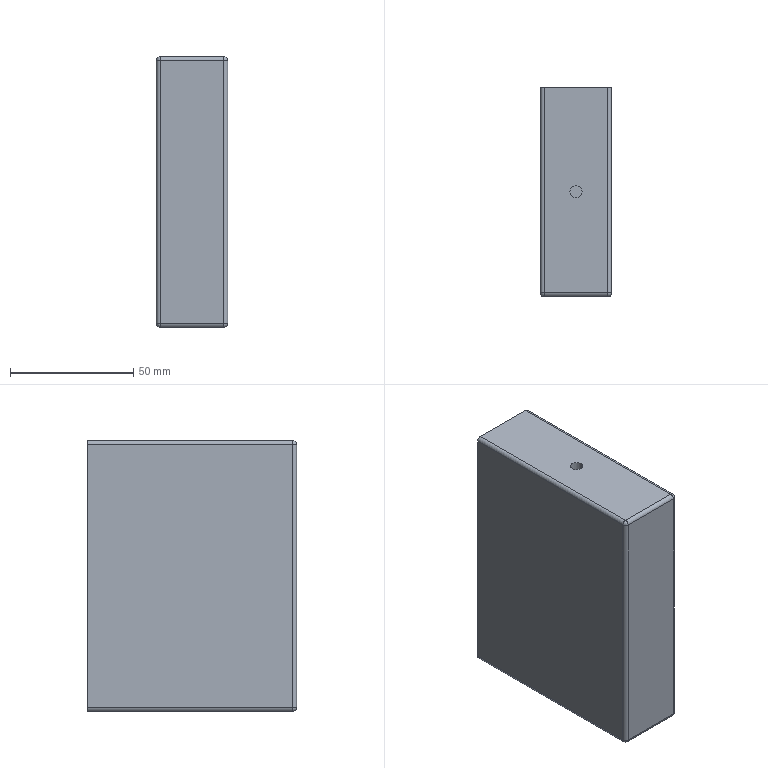Part | SolidWorks | features Extrusion 1, Fillet 1, HoleWzd 1, ICE 1, Shell 1 | 1 solid | 40 faces | box 29 x 85 x 110 mm | volume 26099 mm3 | cylinder 20 | plane 12 | sphere 8 | commonest cylinder face diameters 1 x8 3 x8 5 x2 10 x2
STEP:
#1=CARTESIAN_POINT('',(2.5,0.,51.));
#2=VERTEX_POINT('',#1);
#3=CARTESIAN_POINT('',(-2.5,0.,51.));
#4=VERTEX_POINT('',#3);
#5=CARTESIAN_POINT('',(0.,0.,51.));
#6=DIRECTION('',(0.,0.,-1.));
#7=DIRECTION('',(-1.,0.,0.));
#8=AXIS2_PLACEMENT_3D('',#5,#6,#7);
#9=CIRCLE('',#8,2.5);
#10=EDGE_CURVE('',#2,#4,#9,.T.);
#11=ORIENTED_EDGE('',*,*,#10,.T.);
#12=CARTESIAN_POINT('',(-2.5,0.,55.));
#13=VERTEX_POINT('',#12);
#14=CARTESIAN_POINT('',(-2.5,0.,55.));
#15=DIRECTION('',(0.,0.,1.));
#16=VECTOR('',#15,1000.);
#17=LINE('',#14,#16);
#18=EDGE_CURVE('',#4,#13,#17,.T.);
#19=ORIENTED_EDGE('',*,*,#18,.T.);
#20=CARTESIAN_POINT('',(2.5,0.,55.));
#21=VERTEX_POINT('',#20);
#22=CARTESIAN_POINT('',(0.,0.,55.));
#23=DIRECTION('',(0.,0.,1.));
#24=DIRECTION('',(1.,0.,0.));
#25=AXIS2_PLACEMENT_3D('',#22,#23,#24);
#26=CIRCLE('',#25,2.5);
#27=EDGE_CURVE('',#13,#21,#26,.T.);
#28=ORIENTED_EDGE('',*,*,#27,.T.);
#29=CARTESIAN_POINT('',(2.5,0.,55.));
#30=DIRECTION('',(0.,0.,1.));
#31=VECTOR('',#30,1000.);
#32=LINE('',#29,#31);
#33=EDGE_CURVE('',#2,#21,#32,.T.);
#34=ORIENTED_EDGE('',*,*,#33,.F.);
#35=EDGE_LOOP('',(#11,#19,#28,#34));
#36=FACE_OUTER_BOUND('',#35,.T.);
#37=CARTESIAN_POINT('',(0.,0.,55.));
#38=DIRECTION('',(0.,0.,1.));
#39=DIRECTION('',(1.,0.,0.));
#40=AXIS2_PLACEMENT_3D('',#37,#38,#39);
#41=CYLINDRICAL_SURFACE('',#40,2.5);
#42=ADVANCED_FACE('',(#36),#41,.F.);
#43=CARTESIAN_POINT('',(-5.,0.,51.));
#44=VERTEX_POINT('',#43);
#45=CARTESIAN_POINT('',(5.,0.,51.));
#46=VERTEX_POINT('',#45);
#47=CARTESIAN_POINT('',(0.,0.,51.));
#48=DIRECTION('',(0.,0.,-1.));
#49=DIRECTION('',(-1.,0.,0.));
#50=AXIS2_PLACEMENT_3D('',#47,#48,#49);
#51=CIRCLE('',#50,5.);
#52=EDGE_CURVE('',#44,#46,#51,.T.);
#53=ORIENTED_EDGE('',*,*,#52,.F.);
#54=CARTESIAN_POINT('',(-5.,0.,54.));
#55=VERTEX_POINT('',#54);
#56=CARTESIAN_POINT('',(-5.,0.,51.));
#57=DIRECTION('',(0.,0.,1.));
#58=VECTOR('',#57,1000.);
#59=LINE('',#56,#58);
#60=EDGE_CURVE('',#44,#55,#59,.T.);
#61=ORIENTED_EDGE('',*,*,#60,.T.);
#62=CARTESIAN_POINT('',(5.,0.,54.));
#63=VERTEX_POINT('',#62);
#64=CARTESIAN_POINT('',(0.,0.,54.));
#65=DIRECTION('',(0.,0.,-1.));
#66=DIRECTION('',(-1.,0.,0.));
#67=AXIS2_PLACEMENT_3D('',#64,#65,#66);
#68=CIRCLE('',#67,5.);
#69=EDGE_CURVE('',#55,#63,#68,.T.);
#70=ORIENTED_EDGE('',*,*,#69,.T.);
#71=CARTESIAN_POINT('',(5.,0.,51.));
#72=DIRECTION('',(0.,0.,1.));
#73=VECTOR('',#72,1000.);
#74=LINE('',#71,#73);
#75=EDGE_CURVE('',#46,#63,#74,.T.);
#76=ORIENTED_EDGE('',*,*,#75,.F.);
#77=EDGE_LOOP('',(#53,#61,#70,#76));
#78=FACE_OUTER_BOUND('',#77,.T.);
#79=CARTESIAN_POINT('',(0.,0.,51.));
#80=DIRECTION('',(0.,0.,1.));
#81=DIRECTION('',(1.,0.,0.));
#82=AXIS2_PLACEMENT_3D('',#79,#80,#81);
#83=CYLINDRICAL_SURFACE('',#82,5.);
#84=ADVANCED_FACE('',(#78),#83,.T.);
#85=CARTESIAN_POINT('',(-13.,-41.,54.));
#86=VERTEX_POINT('',#85);
#87=CARTESIAN_POINT('',(13.,-41.,54.));
#88=VERTEX_POINT('',#87);
#89=CARTESIAN_POINT('',(-14.5,-41.,54.));
#90=DIRECTION('',(1.,0.,0.));
#91=VECTOR('',#90,1000.);
#92=LINE('',#89,#91);
#93=EDGE_CURVE('',#86,#88,#92,.T.);
#94=ORIENTED_EDGE('',*,*,#93,.F.);
#95=CARTESIAN_POINT('',(-13.,42.5,54.));
#96=VERTEX_POINT('',#95);
#97=CARTESIAN_POINT('',(-13.,42.5,54.));
#98=DIRECTION('',(0.,-1.,0.));
#99=VECTOR('',#98,1000.);
#100=LINE('',#97,#99);
#101=EDGE_CURVE('',#96,#86,#100,.T.);
#102=ORIENTED_EDGE('',*,*,#101,.F.);
#103=CARTESIAN_POINT('',(13.,42.5,54.));
#104=VERTEX_POINT('',#103);
#105=CARTESIAN_POINT('',(-14.5,42.5,54.));
#106=DIRECTION('',(1.,0.,0.));
#107=VECTOR('',#106,1000.);
#108=LINE('',#105,#107);
#109=EDGE_CURVE('',#96,#104,#108,.T.);
#110=ORIENTED_EDGE('',*,*,#109,.T.);
#111=CARTESIAN_POINT('',(13.,42.5,54.));
#112=DIRECTION('',(0.,1.,0.));
#113=VECTOR('',#112,1000.);
#114=LINE('',#111,#113);
#115=EDGE_CURVE('',#88,#104,#114,.T.);
#116=ORIENTED_EDGE('',*,*,#115,.F.);
#117=EDGE_LOOP('',(#94,#102,#110,#116));
#118=FACE_OUTER_BOUND('',#117,.T.);
#119=CARTESIAN_POINT('',(0.,0.,54.));
#120=DIRECTION('',(0.,0.,-1.));
#121=DIRECTION('',(-1.,0.,0.));
#122=AXIS2_PLACEMENT_3D('',#119,#120,#121);
#123=CIRCLE('',#122,5.);
#124=EDGE_CURVE('',#63,#55,#123,.T.);
#125=ORIENTED_EDGE('',*,*,#124,.F.);
#126=ORIENTED_EDGE('',*,*,#69,.F.);
#127=EDGE_LOOP('',(#125,#126));
#128=FACE_BOUND('',#127,.T.);
#129=CARTESIAN_POINT('',(-14.5,42.5,54.));
#130=DIRECTION('',(0.,0.,-1.));
#131=DIRECTION('',(-1.,0.,0.));
#132=AXIS2_PLACEMENT_3D('',#129,#130,#131);
#133=PLANE('',#132);
#134=ADVANCED_FACE('',(#118,#128),#133,.T.);
#135=CARTESIAN_POINT('',(14.5,-41.,53.5));
#136=VERTEX_POINT('',#135);
#137=CARTESIAN_POINT('',(14.5,-41.,-53.5));
#138=VERTEX_POINT('',#137);
#139=CARTESIAN_POINT('',(14.5,-41.,-55.));
#140=DIRECTION('',(0.,0.,-1.));
#141=VECTOR('',#140,1000.);
#142=LINE('',#139,#141);
#143=EDGE_CURVE('',#136,#138,#142,.T.);
#144=ORIENTED_EDGE('',*,*,#143,.T.);
#145=CARTESIAN_POINT('',(14.5,42.5,-53.5));
#146=VERTEX_POINT('',#145);
#147=CARTESIAN_POINT('',(14.5,42.5,-53.5));
#148=DIRECTION('',(0.,1.,0.));
#149=VECTOR('',#148,1000.);
#150=LINE('',#147,#149);
#151=EDGE_CURVE('',#138,#146,#150,.T.);
#152=ORIENTED_EDGE('',*,*,#151,.T.);
#153=CARTESIAN_POINT('',(14.5,42.5,53.5));
#154=VERTEX_POINT('',#153);
#155=CARTESIAN_POINT('',(14.5,42.5,-55.));
#156=DIRECTION('',(0.,0.,-1.));
#157=VECTOR('',#156,1000.);
#158=LINE('',#155,#157);
#159=EDGE_CURVE('',#154,#146,#158,.T.);
#160=ORIENTED_EDGE('',*,*,#159,.F.);
#161=CARTESIAN_POINT('',(14.5,42.5,53.5));
#162=DIRECTION('',(0.,-1.,0.));
#163=VECTOR('',#162,1000.);
#164=LINE('',#161,#163);
#165=EDGE_CURVE('',#154,#136,#164,.T.);
#166=ORIENTED_EDGE('',*,*,#165,.T.);
#167=EDGE_LOOP('',(#144,#152,#160,#166));
#168=FACE_OUTER_BOUND('',#167,.T.);
#169=CARTESIAN_POINT('',(14.5,42.5,-55.));
#170=DIRECTION('',(-1.,0.,0.));
#171=DIRECTION('',(0.,0.,1.));
#172=AXIS2_PLACEMENT_3D('',#169,#170,#171);
#173=PLANE('',#172);
#174=ADVANCED_FACE('',(#168),#173,.F.);
#175=CARTESIAN_POINT('',(13.,-41.,-55.));
#176=VERTEX_POINT('',#175);
#177=CARTESIAN_POINT('',(-13.,-41.,-55.));
#178=VERTEX_POINT('',#177);
#179=CARTESIAN_POINT('',(-14.5,-41.,-55.));
#180=DIRECTION('',(-1.,0.,0.));
#181=VECTOR('',#180,1000.);
#182=LINE('',#179,#181);
#183=EDGE_CURVE('',#176,#178,#182,.T.);
#184=ORIENTED_EDGE('',*,*,#183,.T.);
#185=CARTESIAN_POINT('',(-13.,42.5,-55.));
#186=VERTEX_POINT('',#185);
#187=CARTESIAN_POINT('',(-13.,42.5,-55.));
#188=DIRECTION('',(0.,1.,0.));
#189=VECTOR('',#188,1000.);
#190=LINE('',#187,#189);
#191=EDGE_CURVE('',#178,#186,#190,.T.);
#192=ORIENTED_EDGE('',*,*,#191,.T.);
#193=CARTESIAN_POINT('',(13.,42.5,-55.));
#194=VERTEX_POINT('',#193);
#195=CARTESIAN_POINT('',(-14.5,42.5,-55.));
#196=DIRECTION('',(-1.,0.,0.));
#197=VECTOR('',#196,1000.);
#198=LINE('',#195,#197);
#199=EDGE_CURVE('',#194,#186,#198,.T.);
#200=ORIENTED_EDGE('',*,*,#199,.F.);
#201=CARTESIAN_POINT('',(13.,42.5,-55.));
#202=DIRECTION('',(0.,-1.,0.));
#203=VECTOR('',#202,1000.);
#204=LINE('',#201,#203);
#205=EDGE_CURVE('',#194,#176,#204,.T.);
#206=ORIENTED_EDGE('',*,*,#205,.T.);
#207=EDGE_LOOP('',(#184,#192,#200,#206));
#208=FACE_OUTER_BOUND('',#207,.T.);
#209=CARTESIAN_POINT('',(-14.5,42.5,-55.));
#210=DIRECTION('',(0.,0.,1.));
#211=DIRECTION('',(1.,0.,0.));
#212=AXIS2_PLACEMENT_3D('',#209,#210,#211);
#213=PLANE('',#212);
#214=ADVANCED_FACE('',(#208),#213,.F.);
#215=CARTESIAN_POINT('',(-14.5,42.5,-53.5));
#216=VERTEX_POINT('',#215);
#217=CARTESIAN_POINT('',(-14.5,42.5,53.5));
#218=VERTEX_POINT('',#217);
#219=CARTESIAN_POINT('',(-14.5,42.5,-55.));
#220=DIRECTION('',(0.,0.,1.));
#221=VECTOR('',#220,1000.);
#222=LINE('',#219,#221);
#223=EDGE_CURVE('',#216,#218,#222,.T.);
#224=ORIENTED_EDGE('',*,*,#223,.F.);
#225=CARTESIAN_POINT('',(-14.5,-41.,-53.5));
#226=VERTEX_POINT('',#225);
#227=CARTESIAN_POINT('',(-14.5,42.5,-53.5));
#228=DIRECTION('',(0.,-1.,0.));
#229=VECTOR('',#228,1000.);
#230=LINE('',#227,#229);
#231=EDGE_CURVE('',#216,#226,#230,.T.);
#232=ORIENTED_EDGE('',*,*,#231,.T.);
#233=CARTESIAN_POINT('',(-14.5,-41.,53.5));
#234=VERTEX_POINT('',#233);
#235=CARTESIAN_POINT('',(-14.5,-41.,-55.));
#236=DIRECTION('',(0.,0.,1.));
#237=VECTOR('',#236,1000.);
#238=LINE('',#235,#237);
#239=EDGE_CURVE('',#226,#234,#238,.T.);
#240=ORIENTED_EDGE('',*,*,#239,.T.);
#241=CARTESIAN_POINT('',(-14.5,42.5,53.5));
#242=DIRECTION('',(0.,1.,0.));
#243=VECTOR('',#242,1000.);
#244=LINE('',#241,#243);
#245=EDGE_CURVE('',#234,#218,#244,.T.);
#246=ORIENTED_EDGE('',*,*,#245,.T.);
#247=EDGE_LOOP('',(#224,#232,#240,#246));
#248=FACE_OUTER_BOUND('',#247,.T.);
#249=CARTESIAN_POINT('',(-14.5,42.5,-55.));
#250=DIRECTION('',(1.,0.,0.));
#251=DIRECTION('',(0.,0.,-1.));
#252=AXIS2_PLACEMENT_3D('',#249,#250,#251);
#253=PLANE('',#252);
#254=ADVANCED_FACE('',(#248),#253,.F.);
#255=CARTESIAN_POINT('',(0.,0.,55.));
#256=DIRECTION('',(0.,0.,1.));
#257=DIRECTION('',(1.,0.,0.));
#258=AXIS2_PLACEMENT_3D('',#255,#256,#257);
#259=CIRCLE('',#258,2.5);
#260=EDGE_CURVE('',#21,#13,#259,.T.);
#261=ORIENTED_EDGE('',*,*,#260,.F.);
#262=ORIENTED_EDGE('',*,*,#27,.F.);
#263=EDGE_LOOP('',(#261,#262));
#264=FACE_BOUND('',#263,.T.);
#265=CARTESIAN_POINT('',(-13.,-41.,55.));
#266=VERTEX_POINT('',#265);
#267=CARTESIAN_POINT('',(13.,-41.,55.));
#268=VERTEX_POINT('',#267);
#269=CARTESIAN_POINT('',(-14.5,-41.,55.));
#270=DIRECTION('',(1.,0.,0.));
#271=VECTOR('',#270,1000.);
#272=LINE('',#269,#271);
#273=EDGE_CURVE('',#266,#268,#272,.T.);
#274=ORIENTED_EDGE('',*,*,#273,.T.);
#275=CARTESIAN_POINT('',(13.,42.5,55.));
#276=VERTEX_POINT('',#275);
#277=CARTESIAN_POINT('',(13.,42.5,55.));
#278=DIRECTION('',(0.,1.,0.));
#279=VECTOR('',#278,1000.);
#280=LINE('',#277,#279);
#281=EDGE_CURVE('',#268,#276,#280,.T.);
#282=ORIENTED_EDGE('',*,*,#281,.T.);
#283=CARTESIAN_POINT('',(-13.,42.5,55.));
#284=VERTEX_POINT('',#283);
#285=CARTESIAN_POINT('',(-14.5,42.5,55.));
#286=DIRECTION('',(1.,0.,0.));
#287=VECTOR('',#286,1000.);
#288=LINE('',#285,#287);
#289=EDGE_CURVE('',#284,#276,#288,.T.);
#290=ORIENTED_EDGE('',*,*,#289,.F.);
#291=CARTESIAN_POINT('',(-13.,42.5,55.));
#292=DIRECTION('',(0.,-1.,0.));
#293=VECTOR('',#292,1000.);
#294=LINE('',#291,#293);
#295=EDGE_CURVE('',#284,#266,#294,.T.);
#296=ORIENTED_EDGE('',*,*,#295,.T.);
#297=EDGE_LOOP('',(#274,#282,#290,#296));
#298=FACE_OUTER_BOUND('',#297,.T.);
#299=CARTESIAN_POINT('',(-14.5,42.5,55.));
#300=DIRECTION('',(0.,0.,-1.));
#301=DIRECTION('',(-1.,0.,0.));
#302=AXIS2_PLACEMENT_3D('',#299,#300,#301);
#303=PLANE('',#302);
#304=ADVANCED_FACE('',(#264,#298),#303,.F.);
#305=CARTESIAN_POINT('',(13.,42.5,-54.));
#306=VERTEX_POINT('',#305);
#307=CARTESIAN_POINT('',(-13.,42.5,-54.));
#308=VERTEX_POINT('',#307);
#309=CARTESIAN_POINT('',(-14.5,42.5,-54.));
#310=DIRECTION('',(-1.,0.,0.));
#311=VECTOR('',#310,1000.);
#312=LINE('',#309,#311);
#313=EDGE_CURVE('',#306,#308,#312,.T.);
#314=ORIENTED_EDGE('',*,*,#313,.F.);
#315=CARTESIAN_POINT('',(13.5,42.5,-53.5));
#316=VERTEX_POINT('',#315);
#317=CARTESIAN_POINT('',(13.,42.5,-53.5));
#318=DIRECTION('',(0.,1.,0.));
#319=DIRECTION('',(0.,0.,1.));
#320=AXIS2_PLACEMENT_3D('',#317,#318,#319);
#321=CIRCLE('',#320,0.5);
#322=EDGE_CURVE('',#316,#306,#321,.T.);
#323=ORIENTED_EDGE('',*,*,#322,.F.);
#324=CARTESIAN_POINT('',(13.5,42.5,53.5));
#325=VERTEX_POINT('',#324);
#326=CARTESIAN_POINT('',(13.5,42.5,-55.));
#327=DIRECTION('',(0.,0.,-1.));
#328=VECTOR('',#327,1000.);
#329=LINE('',#326,#328);
#330=EDGE_CURVE('',#325,#316,#329,.T.);
#331=ORIENTED_EDGE('',*,*,#330,.F.);
#332=CARTESIAN_POINT('',(13.,42.5,53.5));
#333=DIRECTION('',(0.,1.,0.));
#334=DIRECTION('',(0.,0.,1.));
#335=AXIS2_PLACEMENT_3D('',#332,#333,#334);
#336=CIRCLE('',#335,0.5);
#337=EDGE_CURVE('',#104,#325,#336,.T.);
#338=ORIENTED_EDGE('',*,*,#337,.F.);
#339=ORIENTED_EDGE('',*,*,#109,.F.);
#340=CARTESIAN_POINT('',(-13.5,42.5,53.5));
#341=VERTEX_POINT('',#340);
#342=CARTESIAN_POINT('',(-13.,42.5,53.5));
#343=DIRECTION('',(0.,1.,0.));
#344=DIRECTION('',(0.,0.,1.));
#345=AXIS2_PLACEMENT_3D('',#342,#343,#344);
#346=CIRCLE('',#345,0.5);
#347=EDGE_CURVE('',#341,#96,#346,.T.);
#348=ORIENTED_EDGE('',*,*,#347,.F.);
#349=CARTESIAN_POINT('',(-13.5,42.5,-53.5));
#350=VERTEX_POINT('',#349);
#351=CARTESIAN_POINT('',(-13.5,42.5,-55.));
#352=DIRECTION('',(0.,0.,1.));
#353=VECTOR('',#352,1000.);
#354=LINE('',#351,#353);
#355=EDGE_CURVE('',#350,#341,#354,.T.);
#356=ORIENTED_EDGE('',*,*,#355,.F.);
#357=CARTESIAN_POINT('',(-13.,42.5,-53.5));
#358=DIRECTION('',(0.,1.,0.));
#359=DIRECTION('',(0.,0.,1.));
#360=AXIS2_PLACEMENT_3D('',#357,#358,#359);
#361=CIRCLE('',#360,0.5);
#362=EDGE_CURVE('',#308,#350,#361,.T.);
#363=ORIENTED_EDGE('',*,*,#362,.F.);
#364=EDGE_LOOP('',(#314,#323,#331,#338,#339,#348,#356,#363));
#365=FACE_BOUND('',#364,.T.);
#366=ORIENTED_EDGE('',*,*,#199,.T.);
#367=CARTESIAN_POINT('',(-13.,42.5,-53.5));
#368=DIRECTION('',(0.,1.,0.));
#369=DIRECTION('',(0.,0.,1.));
#370=AXIS2_PLACEMENT_3D('',#367,#368,#369);
#371=CIRCLE('',#370,1.5);
#372=EDGE_CURVE('',#186,#216,#371,.T.);
#373=ORIENTED_EDGE('',*,*,#372,.T.);
#374=ORIENTED_EDGE('',*,*,#223,.T.);
#375=CARTESIAN_POINT('',(-13.,42.5,53.5));
#376=DIRECTION('',(0.,1.,0.));
#377=DIRECTION('',(0.,0.,1.));
#378=AXIS2_PLACEMENT_3D('',#375,#376,#377);
#379=CIRCLE('',#378,1.5);
#380=EDGE_CURVE('',#218,#284,#379,.T.);
#381=ORIENTED_EDGE('',*,*,#380,.T.);
#382=ORIENTED_EDGE('',*,*,#289,.T.);
#383=CARTESIAN_POINT('',(13.,42.5,53.5));
#384=DIRECTION('',(0.,1.,0.));
#385=DIRECTION('',(0.,0.,1.));
#386=AXIS2_PLACEMENT_3D('',#383,#384,#385);
#387=CIRCLE('',#386,1.5);
#388=EDGE_CURVE('',#276,#154,#387,.T.);
#389=ORIENTED_EDGE('',*,*,#388,.T.);
#390=ORIENTED_EDGE('',*,*,#159,.T.);
#391=CARTESIAN_POINT('',(13.,42.5,-53.5));
#392=DIRECTION('',(0.,1.,0.));
#393=DIRECTION('',(0.,0.,1.));
#394=AXIS2_PLACEMENT_3D('',#391,#392,#393);
#395=CIRCLE('',#394,1.5);
#396=EDGE_CURVE('',#146,#194,#395,.T.);
#397=ORIENTED_EDGE('',*,*,#396,.T.);
#398=EDGE_LOOP('',(#366,#373,#374,#381,#382,#389,#390,#397));
#399=FACE_OUTER_BOUND('',#398,.T.);
#400=CARTESIAN_POINT('',(0.,42.5,0.));
#401=DIRECTION('',(0.,1.,0.));
#402=DIRECTION('',(0.,0.,1.));
#403=AXIS2_PLACEMENT_3D('',#400,#401,#402);
#404=PLANE('',#403);
#405=ADVANCED_FACE('',(#365,#399),#404,.T.);
#406=CARTESIAN_POINT('',(-13.,-42.5,53.5));
#407=VERTEX_POINT('',#406);
#408=CARTESIAN_POINT('',(-13.,-42.5,-53.5));
#409=VERTEX_POINT('',#408);
#410=CARTESIAN_POINT('',(-13.,-42.5,0.));
#411=DIRECTION('',(0.,0.,-1.));
#412=VECTOR('',#411,1000.);
#413=LINE('',#410,#412);
#414=EDGE_CURVE('',#407,#409,#413,.T.);
#415=ORIENTED_EDGE('',*,*,#414,.T.);
#416=CARTESIAN_POINT('',(13.,-42.5,-53.5));
#417=VERTEX_POINT('',#416);
#418=CARTESIAN_POINT('',(0.,-42.5,-53.5));
#419=DIRECTION('',(1.,0.,0.));
#420=VECTOR('',#419,1000.);
#421=LINE('',#418,#420);
#422=EDGE_CURVE('',#409,#417,#421,.T.);
#423=ORIENTED_EDGE('',*,*,#422,.T.);
#424=CARTESIAN_POINT('',(13.,-42.5,53.5));
#425=VERTEX_POINT('',#424);
#426=CARTESIAN_POINT('',(13.,-42.5,0.));
#427=DIRECTION('',(0.,0.,1.));
#428=VECTOR('',#427,1000.);
#429=LINE('',#426,#428);
#430=EDGE_CURVE('',#417,#425,#429,.T.);
#431=ORIENTED_EDGE('',*,*,#430,.T.);
#432=CARTESIAN_POINT('',(0.,-42.5,53.5));
#433=DIRECTION('',(-1.,0.,0.));
#434=VECTOR('',#433,1000.);
#435=LINE('',#432,#434);
#436=EDGE_CURVE('',#425,#407,#435,.T.);
#437=ORIENTED_EDGE('',*,*,#436,.T.);
#438=EDGE_LOOP('',(#415,#423,#431,#437));
#439=FACE_OUTER_BOUND('',#438,.T.);
#440=CARTESIAN_POINT('',(0.,-42.5,0.));
#441=DIRECTION('',(0.,1.,0.));
#442=DIRECTION('',(0.,0.,1.));
#443=AXIS2_PLACEMENT_3D('',#440,#441,#442);
#444=PLANE('',#443);
#445=ADVANCED_FACE('',(#439),#444,.F.);
#446=ORIENTED_EDGE('',*,*,#388,.F.);
#447=ORIENTED_EDGE('',*,*,#281,.F.);
#448=CARTESIAN_POINT('',(13.,-41.,53.5));
#449=DIRECTION('',(0.,-1.,0.));
#450=DIRECTION('',(0.,0.,-1.));
#451=AXIS2_PLACEMENT_3D('',#448,#449,#450);
#452=CIRCLE('',#451,1.5);
#453=EDGE_CURVE('',#136,#268,#452,.T.);
#454=ORIENTED_EDGE('',*,*,#453,.F.);
#455=ORIENTED_EDGE('',*,*,#165,.F.);
#456=EDGE_LOOP('',(#446,#447,#454,#455));
#457=FACE_OUTER_BOUND('',#456,.T.);
#458=CARTESIAN_POINT('',(13.,42.5,53.5));
#459=DIRECTION('',(0.,-1.,0.));
#460=DIRECTION('',(0.,0.,-1.));
#461=AXIS2_PLACEMENT_3D('',#458,#459,#460);
#462=CYLINDRICAL_SURFACE('',#461,1.5);
#463=ADVANCED_FACE('',(#457),#462,.T.);
#464=ORIENTED_EDGE('',*,*,#380,.F.);
#465=ORIENTED_EDGE('',*,*,#245,.F.);
#466=CARTESIAN_POINT('',(-13.,-41.,53.5));
#467=DIRECTION('',(0.,-1.,0.));
#468=DIRECTION('',(0.,0.,-1.));
#469=AXIS2_PLACEMENT_3D('',#466,#467,#468);
#470=CIRCLE('',#469,1.5);
#471=EDGE_CURVE('',#266,#234,#470,.T.);
#472=ORIENTED_EDGE('',*,*,#471,.F.);
#473=ORIENTED_EDGE('',*,*,#295,.F.);
#474=EDGE_LOOP('',(#464,#465,#472,#473));
#475=FACE_OUTER_BOUND('',#474,.T.);
#476=CARTESIAN_POINT('',(-13.,42.5,53.5));
#477=DIRECTION('',(0.,-1.,0.));
#478=DIRECTION('',(0.,0.,-1.));
#479=AXIS2_PLACEMENT_3D('',#476,#477,#478);
#480=CYLINDRICAL_SURFACE('',#479,1.5);
#481=ADVANCED_FACE('',(#475),#480,.T.);
#482=CARTESIAN_POINT('',(13.,-41.,53.5));
#483=DIRECTION('',(1.,0.,0.));
#484=DIRECTION('',(0.,0.,-1.));
#485=AXIS2_PLACEMENT_3D('',#482,#483,#484);
#486=CIRCLE('',#485,1.5);
#487=EDGE_CURVE('',#268,#425,#486,.T.);
#488=ORIENTED_EDGE('',*,*,#487,.F.);
#489=ORIENTED_EDGE('',*,*,#273,.F.);
#490=CARTESIAN_POINT('',(-13.,-41.,53.5));
#491=DIRECTION('',(-1.,0.,0.));
#492=DIRECTION('',(0.,0.,1.));
#493=AXIS2_PLACEMENT_3D('',#490,#491,#492);
#494=CIRCLE('',#493,1.5);
#495=EDGE_CURVE('',#407,#266,#494,.T.);
#496=ORIENTED_EDGE('',*,*,#495,.F.);
#497=ORIENTED_EDGE('',*,*,#436,.F.);
#498=EDGE_LOOP('',(#488,#489,#496,#497));
#499=FACE_OUTER_BOUND('',#498,.T.);
#500=CARTESIAN_POINT('',(-14.5,-41.,53.5));
#501=DIRECTION('',(1.,0.,0.));
#502=DIRECTION('',(0.,0.,-1.));
#503=AXIS2_PLACEMENT_3D('',#500,#501,#502);
#504=CYLINDRICAL_SURFACE('',#503,1.5);
#505=ADVANCED_FACE('',(#499),#504,.T.);
#506=ORIENTED_EDGE('',*,*,#453,.T.);
#507=ORIENTED_EDGE('',*,*,#487,.T.);
#508=CARTESIAN_POINT('',(13.,-41.,53.5));
#509=DIRECTION('',(0.,0.,-1.));
#510=DIRECTION('',(1.,0.,0.));
#511=AXIS2_PLACEMENT_3D('',#508,#509,#510);
#512=CIRCLE('',#511,1.5);
#513=EDGE_CURVE('',#136,#425,#512,.T.);
#514=ORIENTED_EDGE('',*,*,#513,.F.);
#515=EDGE_LOOP('',(#506,#507,#514));
#516=FACE_OUTER_BOUND('',#515,.T.);
#517=CARTESIAN_POINT('',(13.,-41.,53.5));
#518=DIRECTION('',(0.,1.,0.));
#519=DIRECTION('',(1.,0.,0.));
#520=AXIS2_PLACEMENT_3D('',#517,#518,#519);
#521=SPHERICAL_SURFACE('',#520,1.5);
#522=ADVANCED_FACE('',(#516),#521,.T.);
#523=ORIENTED_EDGE('',*,*,#495,.T.);
#524=ORIENTED_EDGE('',*,*,#471,.T.);
#525=CARTESIAN_POINT('',(-13.,-41.,53.5));
#526=DIRECTION('',(0.,0.,-1.));
#527=DIRECTION('',(1.,0.,0.));
#528=AXIS2_PLACEMENT_3D('',#525,#526,#527);
#529=CIRCLE('',#528,1.5);
#530=EDGE_CURVE('',#407,#234,#529,.T.);
#531=ORIENTED_EDGE('',*,*,#530,.F.);
#532=EDGE_LOOP('',(#523,#524,#531));
#533=FACE_OUTER_BOUND('',#532,.T.);
#534=CARTESIAN_POINT('',(-13.,-41.,53.5));
#535=DIRECTION('',(0.,1.,0.));
#536=DIRECTION('',(1.,0.,0.));
#537=AXIS2_PLACEMENT_3D('',#534,#535,#536);
#538=SPHERICAL_SURFACE('',#537,1.5);
#539=ADVANCED_FACE('',(#533),#538,.T.);
#540=ORIENTED_EDGE('',*,*,#513,.T.);
#541=ORIENTED_EDGE('',*,*,#430,.F.);
#542=CARTESIAN_POINT('',(13.,-41.,-53.5));
#543=DIRECTION('',(0.,0.,-1.));
#544=DIRECTION('',(-1.,0.,0.));
#545=AXIS2_PLACEMENT_3D('',#542,#543,#544);
#546=CIRCLE('',#545,1.5);
#547=EDGE_CURVE('',#138,#417,#546,.T.);
#548=ORIENTED_EDGE('',*,*,#547,.F.);
#549=ORIENTED_EDGE('',*,*,#143,.F.);
#550=EDGE_LOOP('',(#540,#541,#548,#549));
#551=FACE_OUTER_BOUND('',#550,.T.);
#552=CARTESIAN_POINT('',(13.,-41.,-55.));
#553=DIRECTION('',(0.,0.,-1.));
#554=DIRECTION('',(-1.,0.,0.));
#555=AXIS2_PLACEMENT_3D('',#552,#553,#554);
#556=CYLINDRICAL_SURFACE('',#555,1.5);
#557=ADVANCED_FACE('',(#551),#556,.T.);
#558=ORIENTED_EDGE('',*,*,#396,.F.);
#559=ORIENTED_EDGE('',*,*,#151,.F.);
#560=CARTESIAN_POINT('',(13.,-41.,-53.5));
#561=DIRECTION('',(0.,-1.,0.));
#562=DIRECTION('',(0.,0.,-1.));
#563=AXIS2_PLACEMENT_3D('',#560,#561,#562);
#564=CIRCLE('',#563,1.5);
#565=EDGE_CURVE('',#176,#138,#564,.T.);
#566=ORIENTED_EDGE('',*,*,#565,.F.);
#567=ORIENTED_EDGE('',*,*,#205,.F.);
#568=EDGE_LOOP('',(#558,#559,#566,#567));
#569=FACE_OUTER_BOUND('',#568,.T.);
#570=CARTESIAN_POINT('',(13.,42.5,-53.5));
#571=DIRECTION('',(0.,-1.,0.));
#572=DIRECTION('',(0.,0.,-1.));
#573=AXIS2_PLACEMENT_3D('',#570,#571,#572);
#574=CYLINDRICAL_SURFACE('',#573,1.5);
#575=ADVANCED_FACE('',(#569),#574,.T.);
#576=ORIENTED_EDGE('',*,*,#372,.F.);
#577=ORIENTED_EDGE('',*,*,#191,.F.);
#578=CARTESIAN_POINT('',(-13.,-41.,-53.5));
#579=DIRECTION('',(0.,-1.,0.));
#580=DIRECTION('',(0.,0.,-1.));
#581=AXIS2_PLACEMENT_3D('',#578,#579,#580);
#582=CIRCLE('',#581,1.5);
#583=EDGE_CURVE('',#226,#178,#582,.T.);
#584=ORIENTED_EDGE('',*,*,#583,.F.);
#585=ORIENTED_EDGE('',*,*,#231,.F.);
#586=EDGE_LOOP('',(#576,#577,#584,#585));
#587=FACE_OUTER_BOUND('',#586,.T.);
#588=CARTESIAN_POINT('',(-13.,42.5,-53.5));
#589=DIRECTION('',(0.,-1.,0.));
#590=DIRECTION('',(0.,0.,-1.));
#591=AXIS2_PLACEMENT_3D('',#588,#589,#590);
#592=CYLINDRICAL_SURFACE('',#591,1.5);
#593=ADVANCED_FACE('',(#587),#592,.T.);
#594=ORIENTED_EDGE('',*,*,#530,.T.);
#595=ORIENTED_EDGE('',*,*,#239,.F.);
#596=CARTESIAN_POINT('',(-13.,-41.,-53.5));
#597=DIRECTION('',(0.,0.,-1.));
#598=DIRECTION('',(-1.,0.,0.));
#599=AXIS2_PLACEMENT_3D('',#596,#597,#598);
#600=CIRCLE('',#599,1.5);
#601=EDGE_CURVE('',#409,#226,#600,.T.);
#602=ORIENTED_EDGE('',*,*,#601,.F.);
#603=ORIENTED_EDGE('',*,*,#414,.F.);
#604=EDGE_LOOP('',(#594,#595,#602,#603));
#605=FACE_OUTER_BOUND('',#604,.T.);
#606=CARTESIAN_POINT('',(-13.,-41.,-55.));
#607=DIRECTION('',(0.,0.,1.));
#608=DIRECTION('',(1.,0.,0.));
#609=AXIS2_PLACEMENT_3D('',#606,#607,#608);
#610=CYLINDRICAL_SURFACE('',#609,1.5);
#611=ADVANCED_FACE('',(#605),#610,.T.);
#612=ORIENTED_EDGE('',*,*,#565,.T.);
#613=ORIENTED_EDGE('',*,*,#547,.T.);
#614=CARTESIAN_POINT('',(13.,-41.,-53.5));
#615=DIRECTION('',(-1.,0.,0.));
#616=DIRECTION('',(0.,0.,-1.));
#617=AXIS2_PLACEMENT_3D('',#614,#615,#616);
#618=CIRCLE('',#617,1.5);
#619=EDGE_CURVE('',#176,#417,#618,.T.);
#620=ORIENTED_EDGE('',*,*,#619,.F.);
#621=EDGE_LOOP('',(#612,#613,#620));
#622=FACE_OUTER_BOUND('',#621,.T.);
#623=CARTESIAN_POINT('',(13.,-41.,-53.5));
#624=DIRECTION('',(0.,1.,0.));
#625=DIRECTION('',(1.,0.,0.));
#626=AXIS2_PLACEMENT_3D('',#623,#624,#625);
#627=SPHERICAL_SURFACE('',#626,1.5);
#628=ADVANCED_FACE('',(#622),#627,.T.);
#629=ORIENTED_EDGE('',*,*,#601,.T.);
#630=ORIENTED_EDGE('',*,*,#583,.T.);
#631=CARTESIAN_POINT('',(-13.,-41.,-53.5));
#632=DIRECTION('',(1.,0.,0.));
#633=DIRECTION('',(0.,0.,1.));
#634=AXIS2_PLACEMENT_3D('',#631,#632,#633);
#635=CIRCLE('',#634,1.5);
#636=EDGE_CURVE('',#409,#178,#635,.T.);
#637=ORIENTED_EDGE('',*,*,#636,.F.);
#638=EDGE_LOOP('',(#629,#630,#637));
#639=FACE_OUTER_BOUND('',#638,.T.);
#640=CARTESIAN_POINT('',(-13.,-41.,-53.5));
#641=DIRECTION('',(0.,1.,0.));
#642=DIRECTION('',(1.,0.,0.));
#643=AXIS2_PLACEMENT_3D('',#640,#641,#642);
#644=SPHERICAL_SURFACE('',#643,1.5);
#645=ADVANCED_FACE('',(#639),#644,.T.);
#646=ORIENTED_EDGE('',*,*,#619,.T.);
#647=ORIENTED_EDGE('',*,*,#422,.F.);
#648=ORIENTED_EDGE('',*,*,#636,.T.);
#649=ORIENTED_EDGE('',*,*,#183,.F.);
#650=EDGE_LOOP('',(#646,#647,#648,#649));
#651=FACE_OUTER_BOUND('',#650,.T.);
#652=CARTESIAN_POINT('',(-14.5,-41.,-53.5));
#653=DIRECTION('',(-1.,0.,0.));
#654=DIRECTION('',(0.,0.,1.));
#655=AXIS2_PLACEMENT_3D('',#652,#653,#654);
#656=CYLINDRICAL_SURFACE('',#655,1.5);
#657=ADVANCED_FACE('',(#651),#656,.T.);
#658=CARTESIAN_POINT('',(13.5,-41.,53.5));
#659=VERTEX_POINT('',#658);
#660=CARTESIAN_POINT('',(13.5,-41.,-53.5));
#661=VERTEX_POINT('',#660);
#662=CARTESIAN_POINT('',(13.5,-41.,-55.));
#663=DIRECTION('',(0.,0.,-1.));
#664=VECTOR('',#663,1000.);
#665=LINE('',#662,#664);
#666=EDGE_CURVE('',#659,#661,#665,.T.);
#667=ORIENTED_EDGE('',*,*,#666,.F.);
#668=CARTESIAN_POINT('',(13.5,42.5,53.5));
#669=DIRECTION('',(0.,-1.,0.));
#670=VECTOR('',#669,1000.);
#671=LINE('',#668,#670);
#672=EDGE_CURVE('',#325,#659,#671,.T.);
#673=ORIENTED_EDGE('',*,*,#672,.F.);
#674=ORIENTED_EDGE('',*,*,#330,.T.);
#675=CARTESIAN_POINT('',(13.5,42.5,-53.5));
#676=DIRECTION('',(0.,1.,0.));
#677=VECTOR('',#676,1000.);
#678=LINE('',#675,#677);
#679=EDGE_CURVE('',#661,#316,#678,.T.);
#680=ORIENTED_EDGE('',*,*,#679,.F.);
#681=EDGE_LOOP('',(#667,#673,#674,#680));
#682=FACE_OUTER_BOUND('',#681,.T.);
#683=CARTESIAN_POINT('',(13.5,42.5,-55.));
#684=DIRECTION('',(-1.,0.,0.));
#685=DIRECTION('',(0.,0.,1.));
#686=AXIS2_PLACEMENT_3D('',#683,#684,#685);
#687=PLANE('',#686);
#688=ADVANCED_FACE('',(#682),#687,.T.);
#689=CARTESIAN_POINT('',(13.,-41.,-54.));
#690=VERTEX_POINT('',#689);
#691=CARTESIAN_POINT('',(-13.,-41.,-54.));
#692=VERTEX_POINT('',#691);
#693=CARTESIAN_POINT('',(-14.5,-41.,-54.));
#694=DIRECTION('',(-1.,0.,0.));
#695=VECTOR('',#694,1000.);
#696=LINE('',#693,#695);
#697=EDGE_CURVE('',#690,#692,#696,.T.);
#698=ORIENTED_EDGE('',*,*,#697,.F.);
#699=CARTESIAN_POINT('',(13.,42.5,-54.));
#700=DIRECTION('',(0.,-1.,0.));
#701=VECTOR('',#700,1000.);
#702=LINE('',#699,#701);
#703=EDGE_CURVE('',#306,#690,#702,.T.);
#704=ORIENTED_EDGE('',*,*,#703,.F.);
#705=ORIENTED_EDGE('',*,*,#313,.T.);
#706=CARTESIAN_POINT('',(-13.,42.5,-54.));
#707=DIRECTION('',(0.,1.,0.));
#708=VECTOR('',#707,1000.);
#709=LINE('',#706,#708);
#710=EDGE_CURVE('',#692,#308,#709,.T.);
#711=ORIENTED_EDGE('',*,*,#710,.F.);
#712=EDGE_LOOP('',(#698,#704,#705,#711));
#713=FACE_OUTER_BOUND('',#712,.T.);
#714=CARTESIAN_POINT('',(-14.5,42.5,-54.));
#715=DIRECTION('',(0.,0.,1.));
#716=DIRECTION('',(1.,0.,0.));
#717=AXIS2_PLACEMENT_3D('',#714,#715,#716);
#718=PLANE('',#717);
#719=ADVANCED_FACE('',(#713),#718,.T.);
#720=ORIENTED_EDGE('',*,*,#355,.T.);
#721=CARTESIAN_POINT('',(-13.5,-41.,53.5));
#722=VERTEX_POINT('',#721);
#723=CARTESIAN_POINT('',(-13.5,42.5,53.5));
#724=DIRECTION('',(0.,1.,0.));
#725=VECTOR('',#724,1000.);
#726=LINE('',#723,#725);
#727=EDGE_CURVE('',#722,#341,#726,.T.);
#728=ORIENTED_EDGE('',*,*,#727,.F.);
#729=CARTESIAN_POINT('',(-13.5,-41.,-53.5));
#730=VERTEX_POINT('',#729);
#731=CARTESIAN_POINT('',(-13.5,-41.,-55.));
#732=DIRECTION('',(0.,0.,1.));
#733=VECTOR('',#732,1000.);
#734=LINE('',#731,#733);
#735=EDGE_CURVE('',#730,#722,#734,.T.);
#736=ORIENTED_EDGE('',*,*,#735,.F.);
#737=CARTESIAN_POINT('',(-13.5,42.5,-53.5));
#738=DIRECTION('',(0.,-1.,0.));
#739=VECTOR('',#738,1000.);
#740=LINE('',#737,#739);
#741=EDGE_CURVE('',#350,#730,#740,.T.);
#742=ORIENTED_EDGE('',*,*,#741,.F.);
#743=EDGE_LOOP('',(#720,#728,#736,#742));
#744=FACE_OUTER_BOUND('',#743,.T.);
#745=CARTESIAN_POINT('',(-13.5,42.5,-55.));
#746=DIRECTION('',(1.,0.,0.));
#747=DIRECTION('',(0.,0.,-1.));
#748=AXIS2_PLACEMENT_3D('',#745,#746,#747);
#749=PLANE('',#748);
#750=ADVANCED_FACE('',(#744),#749,.T.);
#751=CARTESIAN_POINT('',(-13.,-41.5,53.5));
#752=VERTEX_POINT('',#751);
#753=CARTESIAN_POINT('',(-13.,-41.5,-53.5));
#754=VERTEX_POINT('',#753);
#755=CARTESIAN_POINT('',(-13.,-41.5,0.));
#756=DIRECTION('',(0.,0.,-1.));
#757=VECTOR('',#756,1000.);
#758=LINE('',#755,#757);
#759=EDGE_CURVE('',#752,#754,#758,.T.);
#760=ORIENTED_EDGE('',*,*,#759,.F.);
#761=CARTESIAN_POINT('',(13.,-41.5,53.5));
#762=VERTEX_POINT('',#761);
#763=CARTESIAN_POINT('',(0.,-41.5,53.5));
#764=DIRECTION('',(-1.,0.,0.));
#765=VECTOR('',#764,1000.);
#766=LINE('',#763,#765);
#767=EDGE_CURVE('',#762,#752,#766,.T.);
#768=ORIENTED_EDGE('',*,*,#767,.F.);
#769=CARTESIAN_POINT('',(13.,-41.5,-53.5));
#770=VERTEX_POINT('',#769);
#771=CARTESIAN_POINT('',(13.,-41.5,0.));
#772=DIRECTION('',(0.,0.,1.));
#773=VECTOR('',#772,1000.);
#774=LINE('',#771,#773);
#775=EDGE_CURVE('',#770,#762,#774,.T.);
#776=ORIENTED_EDGE('',*,*,#775,.F.);
#777=CARTESIAN_POINT('',(0.,-41.5,-53.5));
#778=DIRECTION('',(1.,0.,0.));
#779=VECTOR('',#778,1000.);
#780=LINE('',#777,#779);
#781=EDGE_CURVE('',#754,#770,#780,.T.);
#782=ORIENTED_EDGE('',*,*,#781,.F.);
#783=EDGE_LOOP('',(#760,#768,#776,#782));
#784=FACE_OUTER_BOUND('',#783,.T.);
#785=CARTESIAN_POINT('',(0.,-41.5,0.));
#786=DIRECTION('',(0.,1.,0.));
#787=DIRECTION('',(0.,0.,1.));
#788=AXIS2_PLACEMENT_3D('',#785,#786,#787);
#789=PLANE('',#788);
#790=ADVANCED_FACE('',(#784),#789,.T.);
#791=ORIENTED_EDGE('',*,*,#337,.T.);
#792=ORIENTED_EDGE('',*,*,#672,.T.);
#793=CARTESIAN_POINT('',(13.,-41.,53.5));
#794=DIRECTION('',(0.,-1.,0.));
#795=DIRECTION('',(0.,0.,-1.));
#796=AXIS2_PLACEMENT_3D('',#793,#794,#795);
#797=CIRCLE('',#796,0.5);
#798=EDGE_CURVE('',#659,#88,#797,.T.);
#799=ORIENTED_EDGE('',*,*,#798,.T.);
#800=ORIENTED_EDGE('',*,*,#115,.T.);
#801=EDGE_LOOP('',(#791,#792,#799,#800));
#802=FACE_OUTER_BOUND('',#801,.T.);
#803=CARTESIAN_POINT('',(13.,42.5,53.5));
#804=DIRECTION('',(0.,-1.,0.));
#805=DIRECTION('',(0.,0.,-1.));
#806=AXIS2_PLACEMENT_3D('',#803,#804,#805);
#807=CYLINDRICAL_SURFACE('',#806,0.5);
#808=ADVANCED_FACE('',(#802),#807,.F.);
#809=ORIENTED_EDGE('',*,*,#347,.T.);
#810=ORIENTED_EDGE('',*,*,#101,.T.);
#811=CARTESIAN_POINT('',(-13.,-41.,53.5));
#812=DIRECTION('',(0.,-1.,0.));
#813=DIRECTION('',(-1.,0.,0.));
#814=AXIS2_PLACEMENT_3D('',#811,#812,#813);
#815=CIRCLE('',#814,0.5);
#816=EDGE_CURVE('',#86,#722,#815,.T.);
#817=ORIENTED_EDGE('',*,*,#816,.T.);
#818=ORIENTED_EDGE('',*,*,#727,.T.);
#819=EDGE_LOOP('',(#809,#810,#817,#818));
#820=FACE_OUTER_BOUND('',#819,.T.);
#821=CARTESIAN_POINT('',(-13.,42.5,53.5));
#822=DIRECTION('',(0.,-1.,0.));
#823=DIRECTION('',(0.,0.,-1.));
#824=AXIS2_PLACEMENT_3D('',#821,#822,#823);
#825=CYLINDRICAL_SURFACE('',#824,0.5);
#826=ADVANCED_FACE('',(#820),#825,.F.);
#827=CARTESIAN_POINT('',(13.,-41.,53.5));
#828=DIRECTION('',(1.,0.,0.));
#829=DIRECTION('',(0.,-1.,0.));
#830=AXIS2_PLACEMENT_3D('',#827,#828,#829);
#831=CIRCLE('',#830,0.5);
#832=EDGE_CURVE('',#88,#762,#831,.T.);
#833=ORIENTED_EDGE('',*,*,#832,.T.);
#834=ORIENTED_EDGE('',*,*,#767,.T.);
#835=CARTESIAN_POINT('',(-13.,-41.,53.5));
#836=DIRECTION('',(-1.,0.,0.));
#837=DIRECTION('',(0.,-1.,0.));
#838=AXIS2_PLACEMENT_3D('',#835,#836,#837);
#839=CIRCLE('',#838,0.5);
#840=EDGE_CURVE('',#752,#86,#839,.T.);
#841=ORIENTED_EDGE('',*,*,#840,.T.);
#842=ORIENTED_EDGE('',*,*,#93,.T.);
#843=EDGE_LOOP('',(#833,#834,#841,#842));
#844=FACE_OUTER_BOUND('',#843,.T.);
#845=CARTESIAN_POINT('',(-14.5,-41.,53.5));
#846=DIRECTION('',(1.,0.,0.));
#847=DIRECTION('',(0.,0.,-1.));
#848=AXIS2_PLACEMENT_3D('',#845,#846,#847);
#849=CYLINDRICAL_SURFACE('',#848,0.5);
#850=ADVANCED_FACE('',(#844),#849,.F.);
#851=ORIENTED_EDGE('',*,*,#798,.F.);
#852=CARTESIAN_POINT('',(13.,-41.,53.5));
#853=DIRECTION('',(0.,0.,-1.));
#854=DIRECTION('',(-1.,0.,0.));
#855=AXIS2_PLACEMENT_3D('',#852,#853,#854);
#856=CIRCLE('',#855,0.5);
#857=EDGE_CURVE('',#659,#762,#856,.T.);
#858=ORIENTED_EDGE('',*,*,#857,.T.);
#859=ORIENTED_EDGE('',*,*,#832,.F.);
#860=EDGE_LOOP('',(#851,#858,#859));
#861=FACE_OUTER_BOUND('',#860,.T.);
#862=CARTESIAN_POINT('',(13.,-41.,53.5));
#863=DIRECTION('',(0.,1.,0.));
#864=DIRECTION('',(1.,0.,0.));
#865=AXIS2_PLACEMENT_3D('',#862,#863,#864);
#866=SPHERICAL_SURFACE('',#865,0.5);
#867=ADVANCED_FACE('',(#861),#866,.F.);
#868=ORIENTED_EDGE('',*,*,#840,.F.);
#869=CARTESIAN_POINT('',(-13.,-41.,53.5));
#870=DIRECTION('',(0.,0.,-1.));
#871=DIRECTION('',(1.,0.,0.));
#872=AXIS2_PLACEMENT_3D('',#869,#870,#871);
#873=CIRCLE('',#872,0.5);
#874=EDGE_CURVE('',#752,#722,#873,.T.);
#875=ORIENTED_EDGE('',*,*,#874,.T.);
#876=ORIENTED_EDGE('',*,*,#816,.F.);
#877=EDGE_LOOP('',(#868,#875,#876));
#878=FACE_OUTER_BOUND('',#877,.T.);
#879=CARTESIAN_POINT('',(-13.,-41.,53.5));
#880=DIRECTION('',(0.,1.,0.));
#881=DIRECTION('',(1.,0.,0.));
#882=AXIS2_PLACEMENT_3D('',#879,#880,#881);
#883=SPHERICAL_SURFACE('',#882,0.5);
#884=ADVANCED_FACE('',(#878),#883,.F.);
#885=ORIENTED_EDGE('',*,*,#857,.F.);
#886=ORIENTED_EDGE('',*,*,#666,.T.);
#887=CARTESIAN_POINT('',(13.,-41.,-53.5));
#888=DIRECTION('',(0.,0.,-1.));
#889=DIRECTION('',(1.,0.,0.));
#890=AXIS2_PLACEMENT_3D('',#887,#888,#889);
#891=CIRCLE('',#890,0.5);
#892=EDGE_CURVE('',#661,#770,#891,.T.);
#893=ORIENTED_EDGE('',*,*,#892,.T.);
#894=ORIENTED_EDGE('',*,*,#775,.T.);
#895=EDGE_LOOP('',(#885,#886,#893,#894));
#896=FACE_OUTER_BOUND('',#895,.T.);
#897=CARTESIAN_POINT('',(13.,-41.,-55.));
#898=DIRECTION('',(0.,0.,-1.));
#899=DIRECTION('',(-1.,0.,0.));
#900=AXIS2_PLACEMENT_3D('',#897,#898,#899);
#901=CYLINDRICAL_SURFACE('',#900,0.5);
#902=ADVANCED_FACE('',(#896),#901,.F.);
#903=ORIENTED_EDGE('',*,*,#322,.T.);
#904=ORIENTED_EDGE('',*,*,#703,.T.);
#905=CARTESIAN_POINT('',(13.,-41.,-53.5));
#906=DIRECTION('',(0.,-1.,0.));
#907=DIRECTION('',(0.,0.,-1.));
#908=AXIS2_PLACEMENT_3D('',#905,#906,#907);
#909=CIRCLE('',#908,0.5);
#910=EDGE_CURVE('',#690,#661,#909,.T.);
#911=ORIENTED_EDGE('',*,*,#910,.T.);
#912=ORIENTED_EDGE('',*,*,#679,.T.);
#913=EDGE_LOOP('',(#903,#904,#911,#912));
#914=FACE_OUTER_BOUND('',#913,.T.);
#915=CARTESIAN_POINT('',(13.,42.5,-53.5));
#916=DIRECTION('',(0.,-1.,0.));
#917=DIRECTION('',(0.,0.,-1.));
#918=AXIS2_PLACEMENT_3D('',#915,#916,#917);
#919=CYLINDRICAL_SURFACE('',#918,0.5);
#920=ADVANCED_FACE('',(#914),#919,.F.);
#921=ORIENTED_EDGE('',*,*,#362,.T.);
#922=ORIENTED_EDGE('',*,*,#741,.T.);
#923=CARTESIAN_POINT('',(-13.,-41.,-53.5));
#924=DIRECTION('',(0.,-1.,0.));
#925=DIRECTION('',(-1.,0.,0.));
#926=AXIS2_PLACEMENT_3D('',#923,#924,#925);
#927=CIRCLE('',#926,0.5);
#928=EDGE_CURVE('',#730,#692,#927,.T.);
#929=ORIENTED_EDGE('',*,*,#928,.T.);
#930=ORIENTED_EDGE('',*,*,#710,.T.);
#931=EDGE_LOOP('',(#921,#922,#929,#930));
#932=FACE_OUTER_BOUND('',#931,.T.);
#933=CARTESIAN_POINT('',(-13.,42.5,-53.5));
#934=DIRECTION('',(0.,-1.,0.));
#935=DIRECTION('',(0.,0.,-1.));
#936=AXIS2_PLACEMENT_3D('',#933,#934,#935);
#937=CYLINDRICAL_SURFACE('',#936,0.5);
#938=ADVANCED_FACE('',(#932),#937,.F.);
#939=ORIENTED_EDGE('',*,*,#874,.F.);
#940=ORIENTED_EDGE('',*,*,#759,.T.);
#941=CARTESIAN_POINT('',(-13.,-41.,-53.5));
#942=DIRECTION('',(0.,0.,-1.));
#943=DIRECTION('',(1.,0.,0.));
#944=AXIS2_PLACEMENT_3D('',#941,#942,#943);
#945=CIRCLE('',#944,0.5);
#946=EDGE_CURVE('',#754,#730,#945,.T.);
#947=ORIENTED_EDGE('',*,*,#946,.T.);
#948=ORIENTED_EDGE('',*,*,#735,.T.);
#949=EDGE_LOOP('',(#939,#940,#947,#948));
#950=FACE_OUTER_BOUND('',#949,.T.);
#951=CARTESIAN_POINT('',(-13.,-41.,-55.));
#952=DIRECTION('',(0.,0.,1.));
#953=DIRECTION('',(1.,0.,0.));
#954=AXIS2_PLACEMENT_3D('',#951,#952,#953);
#955=CYLINDRICAL_SURFACE('',#954,0.5);
#956=ADVANCED_FACE('',(#950),#955,.F.);
#957=ORIENTED_EDGE('',*,*,#910,.F.);
#958=CARTESIAN_POINT('',(13.,-41.,-53.5));
#959=DIRECTION('',(-1.,0.,0.));
#960=DIRECTION('',(0.,0.,1.));
#961=AXIS2_PLACEMENT_3D('',#958,#959,#960);
#962=CIRCLE('',#961,0.5);
#963=EDGE_CURVE('',#690,#770,#962,.T.);
#964=ORIENTED_EDGE('',*,*,#963,.T.);
#965=ORIENTED_EDGE('',*,*,#892,.F.);
#966=EDGE_LOOP('',(#957,#964,#965));
#967=FACE_OUTER_BOUND('',#966,.T.);
#968=CARTESIAN_POINT('',(13.,-41.,-53.5));
#969=DIRECTION('',(0.,1.,0.));
#970=DIRECTION('',(1.,0.,0.));
#971=AXIS2_PLACEMENT_3D('',#968,#969,#970);
#972=SPHERICAL_SURFACE('',#971,0.5);
#973=ADVANCED_FACE('',(#967),#972,.F.);
#974=ORIENTED_EDGE('',*,*,#946,.F.);
#975=CARTESIAN_POINT('',(-13.,-41.,-53.5));
#976=DIRECTION('',(1.,0.,0.));
#977=DIRECTION('',(0.,0.,1.));
#978=AXIS2_PLACEMENT_3D('',#975,#976,#977);
#979=CIRCLE('',#978,0.5);
#980=EDGE_CURVE('',#754,#692,#979,.T.);
#981=ORIENTED_EDGE('',*,*,#980,.T.);
#982=ORIENTED_EDGE('',*,*,#928,.F.);
#983=EDGE_LOOP('',(#974,#981,#982));
#984=FACE_OUTER_BOUND('',#983,.T.);
#985=CARTESIAN_POINT('',(-13.,-41.,-53.5));
#986=DIRECTION('',(0.,1.,0.));
#987=DIRECTION('',(1.,0.,0.));
#988=AXIS2_PLACEMENT_3D('',#985,#986,#987);
#989=SPHERICAL_SURFACE('',#988,0.5);
#990=ADVANCED_FACE('',(#984),#989,.F.);
#991=ORIENTED_EDGE('',*,*,#963,.F.);
#992=ORIENTED_EDGE('',*,*,#697,.T.);
#993=ORIENTED_EDGE('',*,*,#980,.F.);
#994=ORIENTED_EDGE('',*,*,#781,.T.);
#995=EDGE_LOOP('',(#991,#992,#993,#994));
#996=FACE_OUTER_BOUND('',#995,.T.);
#997=CARTESIAN_POINT('',(-14.5,-41.,-53.5));
#998=DIRECTION('',(-1.,0.,0.));
#999=DIRECTION('',(0.,0.,1.));
#1000=AXIS2_PLACEMENT_3D('',#997,#998,#999);
#1001=CYLINDRICAL_SURFACE('',#1000,0.5);
#1002=ADVANCED_FACE('',(#996),#1001,.F.);
#1003=ORIENTED_EDGE('',*,*,#60,.F.);
#1004=CARTESIAN_POINT('',(0.,0.,51.));
#1005=DIRECTION('',(0.,0.,-1.));
#1006=DIRECTION('',(-1.,0.,0.));
#1007=AXIS2_PLACEMENT_3D('',#1004,#1005,#1006);
#1008=CIRCLE('',#1007,5.);
#1009=EDGE_CURVE('',#46,#44,#1008,.T.);
#1010=ORIENTED_EDGE('',*,*,#1009,.F.);
#1011=ORIENTED_EDGE('',*,*,#75,.T.);
#1012=ORIENTED_EDGE('',*,*,#124,.T.);
#1013=EDGE_LOOP('',(#1003,#1010,#1011,#1012));
#1014=FACE_OUTER_BOUND('',#1013,.T.);
#1015=CARTESIAN_POINT('',(0.,0.,51.));
#1016=DIRECTION('',(0.,0.,1.));
#1017=DIRECTION('',(1.,0.,0.));
#1018=AXIS2_PLACEMENT_3D('',#1015,#1016,#1017);
#1019=CYLINDRICAL_SURFACE('',#1018,5.);
#1020=ADVANCED_FACE('',(#1014),#1019,.T.);
#1021=ORIENTED_EDGE('',*,*,#10,.F.);
#1022=CARTESIAN_POINT('',(0.,0.,51.));
#1023=DIRECTION('',(0.,0.,-1.));
#1024=DIRECTION('',(-1.,0.,0.));
#1025=AXIS2_PLACEMENT_3D('',#1022,#1023,#1024);
#1026=CIRCLE('',#1025,2.5);
#1027=EDGE_CURVE('',#4,#2,#1026,.T.);
#1028=ORIENTED_EDGE('',*,*,#1027,.F.);
#1029=EDGE_LOOP('',(#1021,#1028));
#1030=FACE_BOUND('',#1029,.T.);
#1031=ORIENTED_EDGE('',*,*,#1009,.T.);
#1032=ORIENTED_EDGE('',*,*,#52,.T.);
#1033=EDGE_LOOP('',(#1031,#1032));
#1034=FACE_OUTER_BOUND('',#1033,.T.);
#1035=CARTESIAN_POINT('',(0.,0.,51.));
#1036=DIRECTION('',(0.,0.,-1.));
#1037=DIRECTION('',(-1.,0.,0.));
#1038=AXIS2_PLACEMENT_3D('',#1035,#1036,#1037);
#1039=PLANE('',#1038);
#1040=ADVANCED_FACE('',(#1030,#1034),#1039,.T.);
#1041=ORIENTED_EDGE('',*,*,#18,.F.);
#1042=ORIENTED_EDGE('',*,*,#1027,.T.);
#1043=ORIENTED_EDGE('',*,*,#33,.T.);
#1044=ORIENTED_EDGE('',*,*,#260,.T.);
#1045=EDGE_LOOP('',(#1041,#1042,#1043,#1044));
#1046=FACE_OUTER_BOUND('',#1045,.T.);
#1047=CARTESIAN_POINT('',(0.,0.,55.));
#1048=DIRECTION('',(0.,0.,1.));
#1049=DIRECTION('',(1.,0.,0.));
#1050=AXIS2_PLACEMENT_3D('',#1047,#1048,#1049);
#1051=CYLINDRICAL_SURFACE('',#1050,2.5);
#1052=ADVANCED_FACE('',(#1046),#1051,.F.);
#1053=CLOSED_SHELL('',(#42,#84,#134,#174,#214,#254,#304,#405,#445,#463,#481,#505,#522,#539,#557,#575,#593,#611,#628,#645,#657,#688,#719,#750,#790,#808,#826,#850,#867,#884,#902,#920,#938,#956,#973,#990,#1002,#1020,#1040,#1052));
#1054=MANIFOLD_SOLID_BREP('',#1053);
#1055=CARTESIAN_POINT('',(0.,0.,0.));
#1056=DIRECTION('',(0.,0.,1.));
#1057=DIRECTION('',(1.,0.,0.));
#1058=AXIS2_PLACEMENT_3D('',#1055,#1056,#1057);
#1059=(LENGTH_UNIT()NAMED_UNIT(*)SI_UNIT(.MILLI.,.METRE.));
#1060=UNCERTAINTY_MEASURE_WITH_UNIT(LENGTH_MEASURE(0.00001),#1059,'','');
#1061=(NAMED_UNIT(*)PLANE_ANGLE_UNIT()SI_UNIT($,.RADIAN.));
#1062=(NAMED_UNIT(*)SI_UNIT($,.STERADIAN.)SOLID_ANGLE_UNIT());
#1063=(GEOMETRIC_REPRESENTATION_CONTEXT(3)GLOBAL_UNCERTAINTY_ASSIGNED_CONTEXT((#1060))GLOBAL_UNIT_ASSIGNED_CONTEXT((#1059,#1061,#1062))REPRESENTATION_CONTEXT('',''));
#1064=ADVANCED_BREP_SHAPE_REPRESENTATION('',(#1054,#1058),#1063);